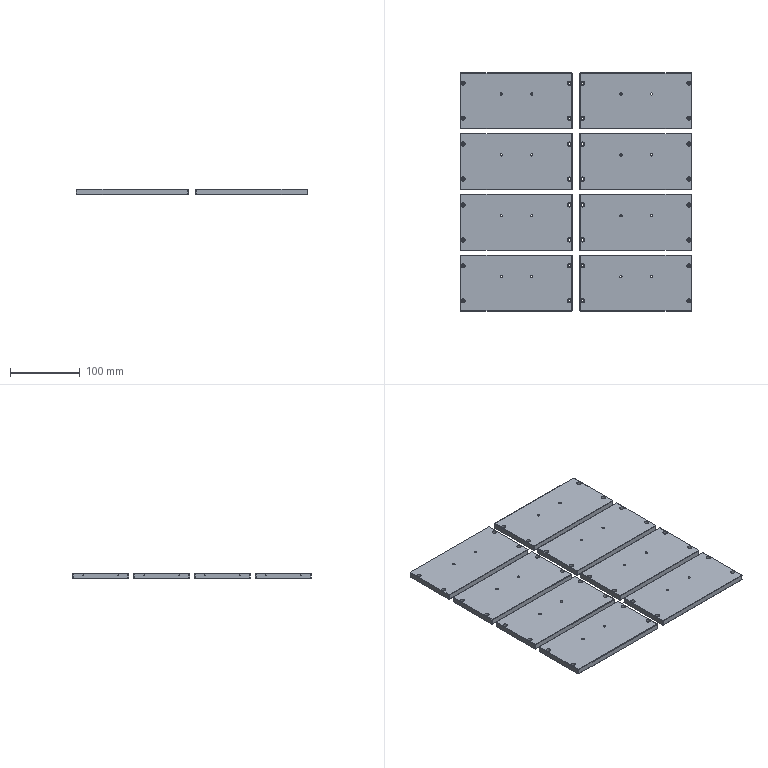Part | 8 solids | 400 faces | box 331 x 341 x 8 mm | volume 812245 mm3 | cylinder 192 | plane 144 | cone 64 | commonest cylinder face diameters 3.5 x64 6 x64 2 x32 3.3 x32